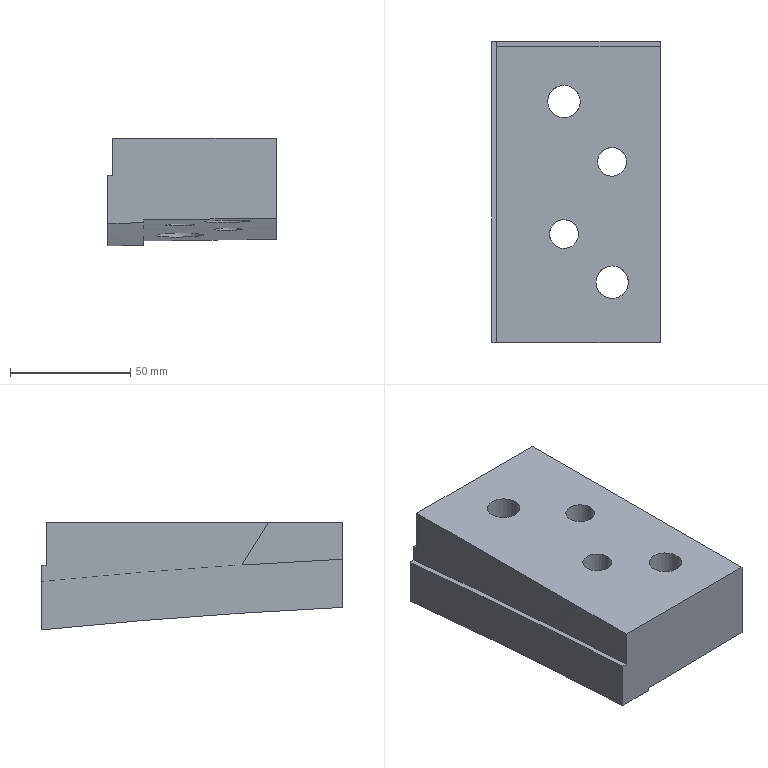Part | NX | features solid 2 | 1 solid | 20 faces | box 70 x 125 x 44.737 mm | volume 296261 mm3 | plane 9 | cylinder 6 | spline 5 | commonest cylinder face diameters 12 x2 13.5 x2 20 x2
STEP:
#1=CARTESIAN_POINT('',(-179.943,183.938,-35.287));
#2=VERTEX_POINT('',#1);
#3=CARTESIAN_POINT('',(-176.967,176.38,-34.573));
#4=CARTESIAN_POINT('',(-181.016,183.824,-35.305));
#5=CARTESIAN_POINT('',(-178.63,191.951,-35.933));
#6=CARTESIAN_POINT('',(-171.182,196.023,-36.198));
#7=CARTESIAN_POINT('',(-163.029,193.617,-35.866));
#8=CARTESIAN_POINT('',(-158.987,186.174,-35.195));
#9=CARTESIAN_POINT('',(-161.361,178.062,-34.509));
#10=CARTESIAN_POINT('',(-168.814,173.976,-34.242));
#11=CARTESIAN_POINT('',(-176.967,176.38,-34.573));
#12=CARTESIAN_POINT('',(-181.016,183.824,-35.305));
#13=CARTESIAN_POINT('',(-178.63,191.951,-35.933));
#14=B_SPLINE_CURVE_WITH_KNOTS('',3,(#3,#4,#5,#6,#7,#8,#9,#10,#11,#12,#13),.UNSPECIFIED.,.T.,.F.,(1,1,1,1,1,1,1,1,1,1,1,1,1,1,1),(-0.02349,-0.01566,-0.00783,0.,0.00783,0.01566,0.02349,0.03132,0.03915,0.04698,0.05481,0.06264,0.07047,0.0783,0.08613),.UNSPECIFIED.);
#15=EDGE_CURVE('',#2,#2,#14,.T.);
#16=ORIENTED_EDGE('',*,*,#15,.F.);
#17=EDGE_LOOP('',(#16));
#18=FACE_BOUND('',#17,.T.);
#19=CARTESIAN_POINT('',(-130.,85.,-28.186));
#20=VERTEX_POINT('',#19);
#21=CARTESIAN_POINT('',(-130.,210.,-36.981));
#22=VERTEX_POINT('',#21);
#23=CARTESIAN_POINT('',(-130.,85.,-28.186));
#24=CARTESIAN_POINT('',(-130.,90.217,-28.433));
#25=CARTESIAN_POINT('',(-130.,100.654,-28.855));
#26=CARTESIAN_POINT('',(-130.,113.697,-29.442));
#27=CARTESIAN_POINT('',(-130.,124.133,-29.882));
#28=CARTESIAN_POINT('',(-130.,131.938,-30.619));
#29=CARTESIAN_POINT('',(-130.,139.759,-31.08));
#30=CARTESIAN_POINT('',(-130.,147.597,-31.331));
#31=CARTESIAN_POINT('',(-130.,155.384,-32.198));
#32=CARTESIAN_POINT('',(-130.,163.186,-32.88));
#33=CARTESIAN_POINT('',(-130.,170.992,-33.525));
#34=CARTESIAN_POINT('',(-130.,181.393,-34.457));
#35=CARTESIAN_POINT('',(-130.,194.4,-35.557));
#36=CARTESIAN_POINT('',(-130.,204.797,-36.538));
#37=CARTESIAN_POINT('',(-130.,210.,-36.981));
#38=B_SPLINE_CURVE_WITH_KNOTS('',3,(#23,#24,#25,#26,#27,#28,#29,#30,#31,#32,#33,#34,#35,#36,#37),.UNSPECIFIED.,.F.,.F.,(4,1,1,1,1,1,1,1,1,1,1,1,4),(0.,0.01567,0.03134,0.03917,0.047,0.05484,0.06267,0.07051,0.07834,0.08617,0.09401,0.1097,0.1253),.UNSPECIFIED.);
#39=EDGE_CURVE('',#20,#22,#38,.T.);
#40=ORIENTED_EDGE('',*,*,#39,.F.);
#41=CARTESIAN_POINT('',(-185.066,85.,-28.984));
#42=VERTEX_POINT('',#41);
#43=CARTESIAN_POINT('',(-185.066,85.,-28.984));
#44=CARTESIAN_POINT('',(-166.712,85.,-28.666));
#45=CARTESIAN_POINT('',(-148.356,85.,-28.396));
#46=CARTESIAN_POINT('',(-130.,85.,-28.186));
#47=B_SPLINE_CURVE_WITH_KNOTS('',3,(#43,#44,#45,#46),.UNSPECIFIED.,.F.,.F.,(4,4),(0.,0.05507),.UNSPECIFIED.);
#48=EDGE_CURVE('',#42,#20,#47,.T.);
#49=ORIENTED_EDGE('',*,*,#48,.F.);
#50=CARTESIAN_POINT('',(-185.059,210.,-37.712));
#51=VERTEX_POINT('',#50);
#52=CARTESIAN_POINT('',(-185.059,210.,-37.712));
#53=CARTESIAN_POINT('',(-185.059,204.796,-37.285));
#54=CARTESIAN_POINT('',(-185.06,197.011,-36.442));
#55=CARTESIAN_POINT('',(-185.06,186.606,-35.6));
#56=CARTESIAN_POINT('',(-185.061,178.806,-34.92));
#57=CARTESIAN_POINT('',(-185.061,171.008,-34.212));
#58=CARTESIAN_POINT('',(-185.062,163.206,-33.565));
#59=CARTESIAN_POINT('',(-185.062,155.404,-32.91));
#60=CARTESIAN_POINT('',(-185.063,148.917,-32.201));
#61=CARTESIAN_POINT('',(-185.063,143.701,-31.915));
#62=CARTESIAN_POINT('',(-185.063,139.78,-31.878));
#63=CARTESIAN_POINT('',(-185.063,135.862,-31.76));
#64=CARTESIAN_POINT('',(-185.064,130.652,-31.347));
#65=CARTESIAN_POINT('',(-185.064,124.146,-30.694));
#66=CARTESIAN_POINT('',(-185.064,116.319,-30.312));
#67=CARTESIAN_POINT('',(-185.065,108.489,-29.983));
#68=CARTESIAN_POINT('',(-185.065,98.05,-29.531));
#69=CARTESIAN_POINT('',(-185.066,90.218,-29.244));
#70=CARTESIAN_POINT('',(-185.066,85.,-28.984));
#71=B_SPLINE_CURVE_WITH_KNOTS('',3,(#52,#53,#54,#55,#56,#57,#58,#59,#60,#61,#62,#63,#64,#65,#66,#67,#68,#69,#70),.UNSPECIFIED.,.F.,.F.,(4,1,1,1,1,1,1,1,1,1,1,1,1,1,1,1,4),(0.1412,0.1569,0.1647,0.1726,0.1804,0.1882,0.196,0.2039,0.2078,0.2117,0.2156,0.2195,0.2273,0.2352,0.243,0.2508,0.2665),.UNSPECIFIED.);
#72=EDGE_CURVE('',#51,#42,#71,.T.);
#73=ORIENTED_EDGE('',*,*,#72,.F.);
#74=CARTESIAN_POINT('',(-130.,210.,-36.981));
#75=CARTESIAN_POINT('',(-148.354,210.,-37.164));
#76=CARTESIAN_POINT('',(-166.707,210.,-37.411));
#77=CARTESIAN_POINT('',(-185.059,210.,-37.712));
#78=B_SPLINE_CURVE_WITH_KNOTS('',3,(#74,#75,#76,#77),.UNSPECIFIED.,.F.,.F.,(4,4),(0.007875,0.06294),.UNSPECIFIED.);
#79=EDGE_CURVE('',#22,#51,#78,.T.);
#80=ORIENTED_EDGE('',*,*,#79,.F.);
#81=EDGE_LOOP('',(#40,#49,#73,#80));
#82=FACE_BOUND('',#81,.T.);
#83=CARTESIAN_POINT('',(-144.006,159.739,-32.722));
#84=VERTEX_POINT('',#83);
#85=CARTESIAN_POINT('',(-145.504,155.098,-32.309));
#86=CARTESIAN_POINT('',(-143.359,159.713,-32.721));
#87=CARTESIAN_POINT('',(-145.094,164.485,-33.138));
#88=CARTESIAN_POINT('',(-149.702,166.645,-33.372));
#89=CARTESIAN_POINT('',(-154.499,164.9,-33.28));
#90=CARTESIAN_POINT('',(-156.639,160.284,-32.927));
#91=CARTESIAN_POINT('',(-154.91,155.521,-32.465));
#92=CARTESIAN_POINT('',(-150.302,153.354,-32.183));
#93=CARTESIAN_POINT('',(-145.504,155.098,-32.309));
#94=CARTESIAN_POINT('',(-143.359,159.713,-32.721));
#95=CARTESIAN_POINT('',(-145.094,164.485,-33.138));
#96=B_SPLINE_CURVE_WITH_KNOTS('',3,(#85,#86,#87,#88,#89,#90,#91,#92,#93,#94,#95),.UNSPECIFIED.,.T.,.F.,(1,1,1,1,1,1,1,1,1,1,1,1,1,1,1),(-0.0141,-0.009397,-0.004698,0.,0.004698,0.009397,0.0141,0.01879,0.02349,0.02819,0.03289,0.03759,0.04229,0.04698,0.05168),.UNSPECIFIED.);
#97=EDGE_CURVE('',#84,#84,#96,.T.);
#98=ORIENTED_EDGE('',*,*,#97,.T.);
#99=EDGE_LOOP('',(#98));
#100=FACE_BOUND('',#99,.T.);
#101=CARTESIAN_POINT('',(-164.006,129.731,-30.876));
#102=VERTEX_POINT('',#101);
#103=CARTESIAN_POINT('',(-165.511,125.091,-30.492));
#104=CARTESIAN_POINT('',(-163.359,129.705,-30.865));
#105=CARTESIAN_POINT('',(-165.087,134.477,-31.306));
#106=CARTESIAN_POINT('',(-169.692,136.644,-31.493));
#107=CARTESIAN_POINT('',(-174.491,134.907,-31.495));
#108=CARTESIAN_POINT('',(-176.639,130.294,-31.149));
#109=CARTESIAN_POINT('',(-174.918,125.53,-30.677));
#110=CARTESIAN_POINT('',(-170.312,123.355,-30.46));
#111=CARTESIAN_POINT('',(-165.511,125.091,-30.492));
#112=CARTESIAN_POINT('',(-163.359,129.705,-30.865));
#113=CARTESIAN_POINT('',(-165.087,134.477,-31.306));
#114=B_SPLINE_CURVE_WITH_KNOTS('',3,(#103,#104,#105,#106,#107,#108,#109,#110,#111,#112,#113),.UNSPECIFIED.,.T.,.F.,(1,1,1,1,1,1,1,1,1,1,1,1,1,1,1),(-0.01409,-0.009395,-0.004697,0.,0.004697,0.009395,0.01409,0.01879,0.02349,0.02818,0.03288,0.03758,0.04228,0.04697,0.05167),.UNSPECIFIED.);
#115=EDGE_CURVE('',#102,#102,#114,.T.);
#116=ORIENTED_EDGE('',*,*,#115,.T.);
#117=EDGE_LOOP('',(#116));
#118=FACE_BOUND('',#117,.T.);
#119=CARTESIAN_POINT('',(-159.944,108.946,-29.606));
#120=VERTEX_POINT('',#119);
#121=CARTESIAN_POINT('',(-156.963,101.377,-29.24));
#122=CARTESIAN_POINT('',(-161.021,108.833,-29.617));
#123=CARTESIAN_POINT('',(-158.617,116.966,-29.93));
#124=CARTESIAN_POINT('',(-151.174,121.019,-30.029));
#125=CARTESIAN_POINT('',(-143.034,118.62,-29.799));
#126=CARTESIAN_POINT('',(-138.983,111.17,-29.425));
#127=CARTESIAN_POINT('',(-141.372,103.047,-29.105));
#128=CARTESIAN_POINT('',(-148.822,98.979,-29.022));
#129=CARTESIAN_POINT('',(-156.963,101.377,-29.24));
#130=CARTESIAN_POINT('',(-161.021,108.833,-29.617));
#131=CARTESIAN_POINT('',(-158.617,116.966,-29.93));
#132=B_SPLINE_CURVE_WITH_KNOTS('',3,(#121,#122,#123,#124,#125,#126,#127,#128,#129,#130,#131),.UNSPECIFIED.,.T.,.F.,(1,1,1,1,1,1,1,1,1,1,1,1,1,1,1),(-0.02346,-0.01564,-0.007819,0.,0.007819,0.01564,0.02346,0.03128,0.0391,0.04692,0.05473,0.06255,0.07037,0.07819,0.08601),.UNSPECIFIED.);
#133=EDGE_CURVE('',#120,#120,#132,.T.);
#134=ORIENTED_EDGE('',*,*,#133,.F.);
#135=EDGE_LOOP('',(#134));
#136=FACE_BOUND('',#135,.T.);
#137=CARTESIAN_POINT('',(-125.164,210.,-36.934));
#138=CARTESIAN_POINT('',(-125.138,208.227,-36.783));
#139=CARTESIAN_POINT('',(-125.034,203.794,-36.406));
#140=CARTESIAN_POINT('',(-125.103,195.358,-35.605));
#141=CARTESIAN_POINT('',(-125.804,184.682,-34.716));
#142=CARTESIAN_POINT('',(-125.853,174.009,-33.744));
#143=CARTESIAN_POINT('',(-126.739,164.665,-32.97));
#144=CARTESIAN_POINT('',(-126.764,155.367,-32.181));
#145=CARTESIAN_POINT('',(-124.796,145.924,-31.099));
#146=CARTESIAN_POINT('',(-129.204,135.731,-30.995));
#147=CARTESIAN_POINT('',(-128.429,126.264,-29.981));
#148=CARTESIAN_POINT('',(-128.955,115.603,-29.504));
#149=CARTESIAN_POINT('',(-129.112,106.237,-29.102));
#150=CARTESIAN_POINT('',(-129.396,95.595,-28.637));
#151=CARTESIAN_POINT('',(-129.537,88.96,-28.368));
#152=CARTESIAN_POINT('',(-129.631,85.,-28.182));
#153=CARTESIAN_POINT('',(-130.684,210.,-36.986));
#154=CARTESIAN_POINT('',(-130.661,208.227,-36.835));
#155=CARTESIAN_POINT('',(-130.564,203.794,-36.459));
#156=CARTESIAN_POINT('',(-130.648,195.358,-35.651));
#157=CARTESIAN_POINT('',(-131.356,184.682,-34.768));
#158=CARTESIAN_POINT('',(-131.419,174.009,-33.796));
#159=CARTESIAN_POINT('',(-132.305,164.665,-33.02));
#160=CARTESIAN_POINT('',(-132.34,155.367,-32.235));
#161=CARTESIAN_POINT('',(-130.411,145.924,-31.149));
#162=CARTESIAN_POINT('',(-134.764,135.731,-31.07));
#163=CARTESIAN_POINT('',(-134.01,126.264,-30.045));
#164=CARTESIAN_POINT('',(-134.538,115.603,-29.561));
#165=CARTESIAN_POINT('',(-134.701,106.237,-29.163));
#166=CARTESIAN_POINT('',(-134.989,95.595,-28.699));
#167=CARTESIAN_POINT('',(-135.133,88.96,-28.432));
#168=CARTESIAN_POINT('',(-135.229,85.,-28.246));
#169=CARTESIAN_POINT('',(-151.145,210.,-37.199));
#170=CARTESIAN_POINT('',(-151.132,208.227,-37.049));
#171=CARTESIAN_POINT('',(-151.065,203.794,-36.675));
#172=CARTESIAN_POINT('',(-151.203,195.358,-35.837));
#173=CARTESIAN_POINT('',(-151.935,184.682,-34.977));
#174=CARTESIAN_POINT('',(-152.049,174.009,-34.003));
#175=CARTESIAN_POINT('',(-152.939,164.665,-33.223));
#176=CARTESIAN_POINT('',(-153.012,155.367,-32.456));
#177=CARTESIAN_POINT('',(-151.223,145.924,-31.351));
#178=CARTESIAN_POINT('',(-155.373,135.731,-31.368));
#179=CARTESIAN_POINT('',(-154.699,126.264,-30.304));
#180=CARTESIAN_POINT('',(-155.234,115.603,-29.795));
#181=CARTESIAN_POINT('',(-155.417,106.237,-29.41));
#182=CARTESIAN_POINT('',(-155.724,95.595,-28.948));
#183=CARTESIAN_POINT('',(-155.877,88.96,-28.69));
#184=CARTESIAN_POINT('',(-155.978,85.,-28.501));
#185=CARTESIAN_POINT('',(-171.603,210.,-37.489));
#186=CARTESIAN_POINT('',(-171.602,208.227,-37.342));
#187=CARTESIAN_POINT('',(-171.565,203.794,-36.974));
#188=CARTESIAN_POINT('',(-171.758,195.358,-36.088));
#189=CARTESIAN_POINT('',(-172.514,184.682,-35.254));
#190=CARTESIAN_POINT('',(-172.68,174.009,-34.276));
#191=CARTESIAN_POINT('',(-173.573,164.665,-33.491));
#192=CARTESIAN_POINT('',(-173.683,155.367,-32.745));
#193=CARTESIAN_POINT('',(-172.035,145.924,-31.619));
#194=CARTESIAN_POINT('',(-175.982,135.731,-31.747));
#195=CARTESIAN_POINT('',(-175.387,126.264,-30.641));
#196=CARTESIAN_POINT('',(-175.929,115.603,-30.109));
#197=CARTESIAN_POINT('',(-176.133,106.237,-29.735));
#198=CARTESIAN_POINT('',(-176.457,95.595,-29.273));
#199=CARTESIAN_POINT('',(-176.619,88.96,-29.027));
#200=CARTESIAN_POINT('',(-176.727,85.,-28.833));
#201=CARTESIAN_POINT('',(-186.542,210.,-37.737));
#202=CARTESIAN_POINT('',(-186.549,208.227,-37.591));
#203=CARTESIAN_POINT('',(-186.534,203.794,-37.227));
#204=CARTESIAN_POINT('',(-186.766,195.358,-36.317));
#205=CARTESIAN_POINT('',(-187.54,184.682,-35.497));
#206=CARTESIAN_POINT('',(-187.743,174.009,-34.519));
#207=CARTESIAN_POINT('',(-188.638,164.665,-33.732));
#208=CARTESIAN_POINT('',(-188.776,155.367,-32.999));
#209=CARTESIAN_POINT('',(-187.231,145.924,-31.866));
#210=CARTESIAN_POINT('',(-191.029,135.731,-32.045));
#211=CARTESIAN_POINT('',(-190.493,126.264,-30.916));
#212=CARTESIAN_POINT('',(-191.04,115.603,-30.37));
#213=CARTESIAN_POINT('',(-191.259,106.237,-30.002));
#214=CARTESIAN_POINT('',(-191.596,95.595,-29.541));
#215=CARTESIAN_POINT('',(-191.765,88.96,-29.301));
#216=CARTESIAN_POINT('',(-191.877,85.,-29.103));
#217=B_SPLINE_SURFACE_WITH_KNOTS('',3,3,((#137,#138,#139,#140,#141,#142,#143,#144,#145,#146,#147,#148,#149,#150,#151,#152),(#153,#154,#155,#156,#157,#158,#159,#160,#161,#162,#163,#164,#165,#166,#167,#168),(#169,#170,#171,#172,#173,#174,#175,#176,#177,#178,#179,#180,#181,#182,#183,#184),(#185,#186,#187,#188,#189,#190,#191,#192,#193,#194,#195,#196,#197,#198,#199,#200),(#201,#202,#203,#204,#205,#206,#207,#208,#209,#210,#211,#212,#213,#214,#215,#216)),.UNSPECIFIED.,.F.,.F.,.F.,(4,1,4),(4,1,1,1,1,1,1,1,1,1,1,1,1,4),(0.6105,0.625,0.6643),(0.5208,0.5312,0.5469,0.5703,0.5938,0.6094,0.625,0.6484,0.6641,0.6875,0.7031,0.7266,0.7422,0.7653),.UNSPECIFIED.);
#218=ADVANCED_FACE('',(#18,#82,#100,#118,#136),#217,.F.);
#219=CARTESIAN_POINT('',(-198.,210.,-13.));
#220=VERTEX_POINT('',#219);
#221=CARTESIAN_POINT('',(-130.,210.,-13.));
#222=VERTEX_POINT('',#221);
#223=CARTESIAN_POINT('',(-198.,210.,-13.));
#224=DIRECTION('',(1.,0.,0.));
#225=VECTOR('',#224,1000.);
#226=LINE('',#223,#225);
#227=EDGE_CURVE('',#220,#222,#226,.T.);
#228=ORIENTED_EDGE('',*,*,#227,.T.);
#229=CARTESIAN_POINT('',(-130.,210.,2.));
#230=DIRECTION('',(0.,0.,1.));
#231=VECTOR('',#230,1000.);
#232=LINE('',#229,#231);
#233=EDGE_CURVE('',#22,#222,#232,.T.);
#234=ORIENTED_EDGE('',*,*,#233,.F.);
#235=ORIENTED_EDGE('',*,*,#79,.T.);
#236=CARTESIAN_POINT('',(-185.059,210.,-39.489));
#237=VERTEX_POINT('',#236);
#238=CARTESIAN_POINT('',(-185.059,210.,-115.));
#239=DIRECTION('',(0.,0.,-1.));
#240=VECTOR('',#239,1000.);
#241=LINE('',#238,#240);
#242=EDGE_CURVE('',#51,#237,#241,.T.);
#243=ORIENTED_EDGE('',*,*,#242,.T.);
#244=CARTESIAN_POINT('',(-200.,210.,-39.737));
#245=VERTEX_POINT('',#244);
#246=CARTESIAN_POINT('',(-200.,210.,-39.737));
#247=CARTESIAN_POINT('',(-195.02,210.,-39.651));
#248=CARTESIAN_POINT('',(-190.039,210.,-39.568));
#249=CARTESIAN_POINT('',(-185.059,210.,-39.489));
#250=B_SPLINE_CURVE_WITH_KNOTS('',3,(#246,#247,#248,#249),.UNSPECIFIED.,.F.,.F.,(4,4),(0.000111,0.01505),.UNSPECIFIED.);
#251=EDGE_CURVE('',#245,#237,#250,.T.);
#252=ORIENTED_EDGE('',*,*,#251,.F.);
#253=CARTESIAN_POINT('',(-200.,210.,-19.737));
#254=VERTEX_POINT('',#253);
#255=CARTESIAN_POINT('',(-200.,210.,-34.243));
#256=DIRECTION('',(0.,0.,1.));
#257=VECTOR('',#256,1000.);
#258=LINE('',#255,#257);
#259=EDGE_CURVE('',#254,#245,#258,.F.);
#260=ORIENTED_EDGE('',*,*,#259,.F.);
#261=CARTESIAN_POINT('',(-198.,210.,-19.737));
#262=VERTEX_POINT('',#261);
#263=CARTESIAN_POINT('',(-200.,210.,-19.737));
#264=CARTESIAN_POINT('',(-199.333,210.,-19.737));
#265=CARTESIAN_POINT('',(-198.667,210.,-19.737));
#266=CARTESIAN_POINT('',(-198.,210.,-19.737));
#267=B_SPLINE_CURVE_WITH_KNOTS('',3,(#263,#264,#265,#266),.UNSPECIFIED.,.F.,.F.,(4,4),(0.00001231,0.002012),.UNSPECIFIED.);
#268=EDGE_CURVE('',#254,#262,#267,.T.);
#269=ORIENTED_EDGE('',*,*,#268,.T.);
#270=CARTESIAN_POINT('',(-198.,210.,2.806));
#271=DIRECTION('',(0.,0.,1.));
#272=VECTOR('',#271,1000.);
#273=LINE('',#270,#272);
#274=EDGE_CURVE('',#262,#220,#273,.T.);
#275=ORIENTED_EDGE('',*,*,#274,.T.);
#276=EDGE_LOOP('',(#228,#234,#235,#243,#252,#260,#269,#275));
#277=FACE_BOUND('',#276,.T.);
#278=CARTESIAN_POINT('',(130.,210.,-37.085));
#279=DIRECTION('',(0.,1.,0.));
#280=DIRECTION('',(0.,0.,1.));
#281=AXIS2_PLACEMENT_3D('',#278,#279,#280);
#282=PLANE('',#281);
#283=ADVANCED_FACE('',(#277),#282,.T.);
#284=CARTESIAN_POINT('',(-130.,85.,5.));
#285=VERTEX_POINT('',#284);
#286=CARTESIAN_POINT('',(-198.,85.,5.));
#287=VERTEX_POINT('',#286);
#288=CARTESIAN_POINT('',(412.414,85.,5.));
#289=DIRECTION('',(-1.,0.,0.));
#290=VECTOR('',#289,1000.);
#291=LINE('',#288,#290);
#292=EDGE_CURVE('',#285,#287,#291,.T.);
#293=ORIENTED_EDGE('',*,*,#292,.T.);
#294=CARTESIAN_POINT('',(-198.,85.,-10.4));
#295=VERTEX_POINT('',#294);
#296=CARTESIAN_POINT('',(-198.,85.,229.6));
#297=DIRECTION('',(0.,0.,1.));
#298=VECTOR('',#297,1000.);
#299=LINE('',#296,#298);
#300=EDGE_CURVE('',#287,#295,#299,.F.);
#301=ORIENTED_EDGE('',*,*,#300,.T.);
#302=CARTESIAN_POINT('',(-200.,85.,-10.4));
#303=VERTEX_POINT('',#302);
#304=CARTESIAN_POINT('',(-198.,85.,-10.4));
#305=CARTESIAN_POINT('',(-198.667,85.,-10.4));
#306=CARTESIAN_POINT('',(-199.333,85.,-10.4));
#307=CARTESIAN_POINT('',(-200.,85.,-10.4));
#308=B_SPLINE_CURVE_WITH_KNOTS('',3,(#304,#305,#306,#307),.UNSPECIFIED.,.F.,.F.,(4,4),(0.,1.),.UNSPECIFIED.);
#309=EDGE_CURVE('',#303,#295,#308,.F.);
#310=ORIENTED_EDGE('',*,*,#309,.F.);
#311=CARTESIAN_POINT('',(-200.,85.,-30.4));
#312=VERTEX_POINT('',#311);
#313=CARTESIAN_POINT('',(-200.,85.,-36.84));
#314=DIRECTION('',(0.,0.,1.));
#315=VECTOR('',#314,1000.);
#316=LINE('',#313,#315);
#317=EDGE_CURVE('',#303,#312,#316,.F.);
#318=ORIENTED_EDGE('',*,*,#317,.T.);
#319=CARTESIAN_POINT('',(-185.066,85.,-30.16));
#320=VERTEX_POINT('',#319);
#321=CARTESIAN_POINT('',(-200.,85.,-30.4));
#322=CARTESIAN_POINT('',(-195.022,85.,-30.317));
#323=CARTESIAN_POINT('',(-190.044,85.,-30.237));
#324=CARTESIAN_POINT('',(-185.066,85.,-30.16));
#325=B_SPLINE_CURVE_WITH_KNOTS('',3,(#321,#322,#323,#324),.UNSPECIFIED.,.F.,.F.,(4,4),(0.0001508,0.01509),.UNSPECIFIED.);
#326=EDGE_CURVE('',#312,#320,#325,.T.);
#327=ORIENTED_EDGE('',*,*,#326,.T.);
#328=CARTESIAN_POINT('',(-185.066,85.,-115.));
#329=DIRECTION('',(0.,0.,-1.));
#330=VECTOR('',#329,1000.);
#331=LINE('',#328,#330);
#332=EDGE_CURVE('',#42,#320,#331,.T.);
#333=ORIENTED_EDGE('',*,*,#332,.F.);
#334=ORIENTED_EDGE('',*,*,#48,.T.);
#335=CARTESIAN_POINT('',(-130.,85.,0.505));
#336=DIRECTION('',(0.,0.,-1.));
#337=VECTOR('',#336,1000.);
#338=LINE('',#335,#337);
#339=EDGE_CURVE('',#285,#20,#338,.T.);
#340=ORIENTED_EDGE('',*,*,#339,.F.);
#341=EDGE_LOOP('',(#293,#301,#310,#318,#327,#333,#334,#340));
#342=FACE_BOUND('',#341,.T.);
#343=CARTESIAN_POINT('',(412.414,85.,0.505));
#344=DIRECTION('',(0.,1.,0.));
#345=DIRECTION('',(0.,0.,1.));
#346=AXIS2_PLACEMENT_3D('',#343,#344,#345);
#347=PLANE('',#346);
#348=ADVANCED_FACE('',(#342),#347,.F.);
#349=CARTESIAN_POINT('',(-156.75,110.,5.));
#350=VERTEX_POINT('',#349);
#351=CARTESIAN_POINT('',(-150.,110.,5.));
#352=DIRECTION('',(0.,0.,-1.));
#353=DIRECTION('',(-1.,0.,0.));
#354=AXIS2_PLACEMENT_3D('',#351,#352,#353);
#355=CIRCLE('',#354,6.75);
#356=EDGE_CURVE('',#350,#350,#355,.F.);
#357=ORIENTED_EDGE('',*,*,#356,.F.);
#358=EDGE_LOOP('',(#357));
#359=FACE_BOUND('',#358,.T.);
#360=CARTESIAN_POINT('',(-176.,130.,5.));
#361=VERTEX_POINT('',#360);
#362=CARTESIAN_POINT('',(-170.,130.,5.));
#363=DIRECTION('',(0.,0.,-1.));
#364=DIRECTION('',(-1.,0.,0.));
#365=AXIS2_PLACEMENT_3D('',#362,#363,#364);
#366=CIRCLE('',#365,6.);
#367=EDGE_CURVE('',#361,#361,#366,.F.);
#368=ORIENTED_EDGE('',*,*,#367,.F.);
#369=EDGE_LOOP('',(#368));
#370=FACE_BOUND('',#369,.T.);
#371=CARTESIAN_POINT('',(-156.,160.,5.));
#372=VERTEX_POINT('',#371);
#373=CARTESIAN_POINT('',(-150.,160.,5.));
#374=DIRECTION('',(0.,0.,-1.));
#375=DIRECTION('',(-1.,0.,0.));
#376=AXIS2_PLACEMENT_3D('',#373,#374,#375);
#377=CIRCLE('',#376,6.);
#378=EDGE_CURVE('',#372,#372,#377,.F.);
#379=ORIENTED_EDGE('',*,*,#378,.F.);
#380=EDGE_LOOP('',(#379));
#381=FACE_BOUND('',#380,.T.);
#382=CARTESIAN_POINT('',(-176.75,185.,5.));
#383=VERTEX_POINT('',#382);
#384=CARTESIAN_POINT('',(-170.,185.,5.));
#385=DIRECTION('',(0.,0.,-1.));
#386=DIRECTION('',(-1.,0.,0.));
#387=AXIS2_PLACEMENT_3D('',#384,#385,#386);
#388=CIRCLE('',#387,6.75);
#389=EDGE_CURVE('',#383,#383,#388,.F.);
#390=ORIENTED_EDGE('',*,*,#389,.F.);
#391=EDGE_LOOP('',(#390));
#392=FACE_BOUND('',#391,.T.);
#393=CARTESIAN_POINT('',(-198.,208.,5.));
#394=VERTEX_POINT('',#393);
#395=CARTESIAN_POINT('',(-130.,208.,5.));
#396=VERTEX_POINT('',#395);
#397=CARTESIAN_POINT('',(-198.,208.,5.));
#398=DIRECTION('',(1.,0.,0.));
#399=VECTOR('',#398,1000.);
#400=LINE('',#397,#399);
#401=EDGE_CURVE('',#394,#396,#400,.T.);
#402=ORIENTED_EDGE('',*,*,#401,.F.);
#403=CARTESIAN_POINT('',(-198.,85.,5.));
#404=CARTESIAN_POINT('',(-197.999,126.,5.));
#405=CARTESIAN_POINT('',(-198.,167.,5.));
#406=CARTESIAN_POINT('',(-198.,208.,5.));
#407=B_SPLINE_CURVE_WITH_KNOTS('',3,(#403,#404,#405,#406),.UNSPECIFIED.,.F.,.F.,(4,4),(1.013,1.136),.UNSPECIFIED.);
#408=EDGE_CURVE('',#394,#287,#407,.F.);
#409=ORIENTED_EDGE('',*,*,#408,.T.);
#410=ORIENTED_EDGE('',*,*,#292,.F.);
#411=CARTESIAN_POINT('',(-130.,0.,5.));
#412=DIRECTION('',(0.,-1.,0.));
#413=VECTOR('',#412,1000.);
#414=LINE('',#411,#413);
#415=EDGE_CURVE('',#396,#285,#414,.T.);
#416=ORIENTED_EDGE('',*,*,#415,.F.);
#417=EDGE_LOOP('',(#402,#409,#410,#416));
#418=FACE_BOUND('',#417,.T.);
#419=CARTESIAN_POINT('',(0.,0.,5.));
#420=DIRECTION('',(0.,0.,1.));
#421=DIRECTION('',(-1.,0.,0.));
#422=AXIS2_PLACEMENT_3D('',#419,#420,#421);
#423=PLANE('',#422);
#424=ADVANCED_FACE('',(#359,#370,#381,#392,#418),#423,.T.);
#425=ORIENTED_EDGE('',*,*,#72,.T.);
#426=ORIENTED_EDGE('',*,*,#332,.T.);
#427=CARTESIAN_POINT('',(-185.059,210.,-39.489));
#428=CARTESIAN_POINT('',(-185.061,168.429,-35.293));
#429=CARTESIAN_POINT('',(-185.064,126.732,-32.197));
#430=CARTESIAN_POINT('',(-185.066,85.,-30.16));
#431=B_SPLINE_CURVE_WITH_KNOTS('',3,(#427,#428,#429,#430),.UNSPECIFIED.,.F.,.F.,(4,4),(0.2096,0.335),.UNSPECIFIED.);
#432=EDGE_CURVE('',#237,#320,#431,.T.);
#433=ORIENTED_EDGE('',*,*,#432,.F.);
#434=ORIENTED_EDGE('',*,*,#242,.F.);
#435=EDGE_LOOP('',(#425,#426,#433,#434));
#436=FACE_BOUND('',#435,.T.);
#437=CARTESIAN_POINT('',(-185.071,-2.633,-115.));
#438=DIRECTION('',(1.,-0.00005855,0.));
#439=DIRECTION('',(-0.00005855,-1.,0.));
#440=AXIS2_PLACEMENT_3D('',#437,#438,#439);
#441=PLANE('',#440);
#442=ADVANCED_FACE('',(#436),#441,.T.);
#443=ORIENTED_EDGE('',*,*,#251,.T.);
#444=ORIENTED_EDGE('',*,*,#432,.T.);
#445=ORIENTED_EDGE('',*,*,#326,.F.);
#446=CARTESIAN_POINT('',(-200.,85.,-30.4));
#447=CARTESIAN_POINT('',(-199.999,126.748,-32.44));
#448=CARTESIAN_POINT('',(-200.,168.419,-35.536));
#449=CARTESIAN_POINT('',(-200.,210.,-39.737));
#450=B_SPLINE_CURVE_WITH_KNOTS('',3,(#446,#447,#448,#449),.UNSPECIFIED.,.F.,.F.,(4,4),(0.06314,0.1885),.UNSPECIFIED.);
#451=EDGE_CURVE('',#312,#245,#450,.T.);
#452=ORIENTED_EDGE('',*,*,#451,.T.);
#453=EDGE_LOOP('',(#443,#444,#445,#452));
#454=FACE_BOUND('',#453,.T.);
#455=CARTESIAN_POINT('',(-200.09,210.782,-39.817));
#456=CARTESIAN_POINT('',(-196.307,210.774,-39.751));
#457=CARTESIAN_POINT('',(-192.525,210.766,-39.687));
#458=CARTESIAN_POINT('',(-188.743,210.759,-39.624));
#459=CARTESIAN_POINT('',(-184.961,210.752,-39.564));
#460=CARTESIAN_POINT('',(-200.093,179.075,-36.604));
#461=CARTESIAN_POINT('',(-196.311,179.067,-36.538));
#462=CARTESIAN_POINT('',(-192.529,179.06,-36.475));
#463=CARTESIAN_POINT('',(-188.746,179.052,-36.413));
#464=CARTESIAN_POINT('',(-184.964,179.045,-36.353));
#465=CARTESIAN_POINT('',(-200.097,147.424,-33.968));
#466=CARTESIAN_POINT('',(-196.315,147.416,-33.904));
#467=CARTESIAN_POINT('',(-192.532,147.409,-33.841));
#468=CARTESIAN_POINT('',(-188.75,147.402,-33.779));
#469=CARTESIAN_POINT('',(-184.967,147.394,-33.72));
#470=CARTESIAN_POINT('',(-200.101,115.819,-31.898));
#471=CARTESIAN_POINT('',(-196.319,115.812,-31.834));
#472=CARTESIAN_POINT('',(-192.536,115.804,-31.771));
#473=CARTESIAN_POINT('',(-188.754,115.797,-31.711));
#474=CARTESIAN_POINT('',(-184.971,115.79,-31.652));
#475=CARTESIAN_POINT('',(-200.107,84.252,-30.366));
#476=CARTESIAN_POINT('',(-196.325,84.244,-30.302));
#477=CARTESIAN_POINT('',(-192.542,84.237,-30.24));
#478=CARTESIAN_POINT('',(-188.759,84.23,-30.18));
#479=CARTESIAN_POINT('',(-184.977,84.223,-30.121));
#480=B_SPLINE_SURFACE_WITH_KNOTS('',4,4,((#455,#456,#457,#458,#459),(#460,#461,#462,#463,#464),(#465,#466,#467,#468,#469),(#470,#471,#472,#473,#474),(#475,#476,#477,#478,#479)),.UNSPECIFIED.,.F.,.F.,.F.,(5,5),(5,5),(0.517,0.7098),(0.5564,0.5748),.PIECEWISE_BEZIER_KNOTS.);
#481=ADVANCED_FACE('',(#454),#480,.F.);
#482=CARTESIAN_POINT('',(-200.,85.,-10.4));
#483=CARTESIAN_POINT('',(-199.999,126.738,-12.439));
#484=CARTESIAN_POINT('',(-200.,168.424,-15.537));
#485=CARTESIAN_POINT('',(-200.,210.,-19.737));
#486=B_SPLINE_CURVE_WITH_KNOTS('',3,(#482,#483,#484,#485),.UNSPECIFIED.,.F.,.F.,(4,4),(0.,0.1254),.UNSPECIFIED.);
#487=EDGE_CURVE('',#303,#254,#486,.T.);
#488=ORIENTED_EDGE('',*,*,#487,.F.);
#489=ORIENTED_EDGE('',*,*,#309,.T.);
#490=CARTESIAN_POINT('',(-198.,210.,-19.737));
#491=CARTESIAN_POINT('',(-198.,168.419,-15.537));
#492=CARTESIAN_POINT('',(-197.999,126.751,-12.44));
#493=CARTESIAN_POINT('',(-198.,85.,-10.4));
#494=B_SPLINE_CURVE_WITH_KNOTS('',3,(#490,#491,#492,#493),.UNSPECIFIED.,.F.,.F.,(4,4),(0.5298,1.),.UNSPECIFIED.);
#495=EDGE_CURVE('',#295,#262,#494,.F.);
#496=ORIENTED_EDGE('',*,*,#495,.T.);
#497=ORIENTED_EDGE('',*,*,#268,.F.);
#498=EDGE_LOOP('',(#488,#489,#496,#497));
#499=FACE_BOUND('',#498,.T.);
#500=CARTESIAN_POINT('',(-198.,85.,-10.4));
#501=CARTESIAN_POINT('',(-197.999,126.751,-12.44));
#502=CARTESIAN_POINT('',(-198.,168.419,-15.537));
#503=CARTESIAN_POINT('',(-198.,210.,-19.737));
#504=CARTESIAN_POINT('',(-200.,85.,-10.4));
#505=CARTESIAN_POINT('',(-199.999,126.751,-12.44));
#506=CARTESIAN_POINT('',(-200.,168.419,-15.537));
#507=CARTESIAN_POINT('',(-200.,210.,-19.737));
#508=CARTESIAN_POINT('',(-200.012,85.,-10.4));
#509=CARTESIAN_POINT('',(-200.012,126.751,-12.44));
#510=CARTESIAN_POINT('',(-200.012,168.419,-15.537));
#511=CARTESIAN_POINT('',(-200.012,210.,-19.737));
#512=B_SPLINE_SURFACE_WITH_KNOTS('',1,3,((#500,#501,#502,#503),(#504,#505,#506,#507),(#508,#509,#510,#511)),.RULED_SURF.,.F.,.F.,.F.,(2,1,2),(4,4),(0.,1.,1.006),(0.,0.4702),.PIECEWISE_BEZIER_KNOTS.);
#513=ADVANCED_FACE('',(#499),#512,.F.);
#514=ORIENTED_EDGE('',*,*,#259,.T.);
#515=ORIENTED_EDGE('',*,*,#451,.F.);
#516=ORIENTED_EDGE('',*,*,#317,.F.);
#517=ORIENTED_EDGE('',*,*,#487,.T.);
#518=EDGE_LOOP('',(#514,#515,#516,#517));
#519=FACE_BOUND('',#518,.T.);
#520=CARTESIAN_POINT('',(-200.,210.,-39.913));
#521=CARTESIAN_POINT('',(-200.,210.,-10.224));
#522=CARTESIAN_POINT('',(-200.,168.333,-39.913));
#523=CARTESIAN_POINT('',(-200.,168.333,-10.224));
#524=CARTESIAN_POINT('',(-199.999,126.667,-39.913));
#525=CARTESIAN_POINT('',(-199.999,126.667,-10.224));
#526=CARTESIAN_POINT('',(-200.,85.,-39.913));
#527=CARTESIAN_POINT('',(-200.,85.,-10.224));
#528=B_SPLINE_SURFACE_WITH_KNOTS('',3,1,((#520,#521),(#522,#523),(#524,#525),(#526,#527)),.SURF_OF_LINEAR_EXTRUSION.,.F.,.F.,.F.,(4,4),(2,2),(0.8605,0.9303),(0.,1.),.PIECEWISE_BEZIER_KNOTS.);
#529=ADVANCED_FACE('',(#519),#528,.T.);
#530=CARTESIAN_POINT('',(-198.,208.,-13.));
#531=VERTEX_POINT('',#530);
#532=CARTESIAN_POINT('',(-198.,210.,-13.));
#533=DIRECTION('',(0.,-1.,0.));
#534=VECTOR('',#533,1000.);
#535=LINE('',#532,#534);
#536=EDGE_CURVE('',#220,#531,#535,.T.);
#537=ORIENTED_EDGE('',*,*,#536,.F.);
#538=ORIENTED_EDGE('',*,*,#274,.F.);
#539=ORIENTED_EDGE('',*,*,#495,.F.);
#540=ORIENTED_EDGE('',*,*,#300,.F.);
#541=ORIENTED_EDGE('',*,*,#408,.F.);
#542=CARTESIAN_POINT('',(-198.,208.,7.));
#543=DIRECTION('',(0.,0.,-1.));
#544=VECTOR('',#543,1000.);
#545=LINE('',#542,#544);
#546=EDGE_CURVE('',#394,#531,#545,.T.);
#547=ORIENTED_EDGE('',*,*,#546,.T.);
#548=EDGE_LOOP('',(#537,#538,#539,#540,#541,#547));
#549=FACE_BOUND('',#548,.T.);
#550=CARTESIAN_POINT('',(-198.,85.,-10.4));
#551=CARTESIAN_POINT('',(-198.,85.,14.282));
#552=CARTESIAN_POINT('',(-197.999,126.999,-12.452));
#553=CARTESIAN_POINT('',(-197.999,126.999,12.231));
#554=CARTESIAN_POINT('',(-198.,168.919,-15.573));
#555=CARTESIAN_POINT('',(-198.,168.919,9.109));
#556=CARTESIAN_POINT('',(-198.,210.748,-19.812));
#557=CARTESIAN_POINT('',(-198.,210.748,4.87));
#558=B_SPLINE_SURFACE_WITH_KNOTS('',3,1,((#550,#551),(#552,#553),(#554,#555),(#556,#557)),.SURF_OF_LINEAR_EXTRUSION.,.F.,.F.,.F.,(4,4),(2,2),(0.,0.473),(0.,1.),.PIECEWISE_BEZIER_KNOTS.);
#559=ADVANCED_FACE('',(#549),#558,.F.);
#560=CARTESIAN_POINT('',(-130.,208.,-13.));
#561=VERTEX_POINT('',#560);
#562=CARTESIAN_POINT('',(-130.,208.,7.));
#563=DIRECTION('',(0.,0.,-1.));
#564=VECTOR('',#563,1000.);
#565=LINE('',#562,#564);
#566=EDGE_CURVE('',#396,#561,#565,.T.);
#567=ORIENTED_EDGE('',*,*,#566,.F.);
#568=ORIENTED_EDGE('',*,*,#415,.T.);
#569=ORIENTED_EDGE('',*,*,#339,.T.);
#570=ORIENTED_EDGE('',*,*,#39,.T.);
#571=ORIENTED_EDGE('',*,*,#233,.T.);
#572=CARTESIAN_POINT('',(-130.,210.,-13.));
#573=DIRECTION('',(0.,-1.,0.));
#574=VECTOR('',#573,1000.);
#575=LINE('',#572,#574);
#576=EDGE_CURVE('',#222,#561,#575,.T.);
#577=ORIENTED_EDGE('',*,*,#576,.T.);
#578=EDGE_LOOP('',(#567,#568,#569,#570,#571,#577));
#579=FACE_BOUND('',#578,.T.);
#580=CARTESIAN_POINT('',(-130.,0.,2.));
#581=DIRECTION('',(-1.,0.,0.));
#582=DIRECTION('',(0.,0.,-1.));
#583=AXIS2_PLACEMENT_3D('',#580,#581,#582);
#584=PLANE('',#583);
#585=ADVANCED_FACE('',(#579),#584,.F.);
#586=ORIENTED_EDGE('',*,*,#576,.F.);
#587=ORIENTED_EDGE('',*,*,#227,.F.);
#588=ORIENTED_EDGE('',*,*,#536,.T.);
#589=CARTESIAN_POINT('',(-198.,208.,-13.));
#590=DIRECTION('',(-1.,0.,0.));
#591=VECTOR('',#590,1000.);
#592=LINE('',#589,#591);
#593=EDGE_CURVE('',#531,#561,#592,.F.);
#594=ORIENTED_EDGE('',*,*,#593,.T.);
#595=EDGE_LOOP('',(#586,#587,#588,#594));
#596=FACE_BOUND('',#595,.T.);
#597=CARTESIAN_POINT('',(-198.,210.,-13.));
#598=DIRECTION('',(0.,0.,1.));
#599=DIRECTION('',(1.,0.,0.));
#600=AXIS2_PLACEMENT_3D('',#597,#598,#599);
#601=PLANE('',#600);
#602=ADVANCED_FACE('',(#596),#601,.T.);
#603=ORIENTED_EDGE('',*,*,#593,.F.);
#604=ORIENTED_EDGE('',*,*,#546,.F.);
#605=ORIENTED_EDGE('',*,*,#401,.T.);
#606=ORIENTED_EDGE('',*,*,#566,.T.);
#607=EDGE_LOOP('',(#603,#604,#605,#606));
#608=FACE_BOUND('',#607,.T.);
#609=CARTESIAN_POINT('',(-198.,208.,7.));
#610=DIRECTION('',(0.,-1.,0.));
#611=DIRECTION('',(0.,0.,-1.));
#612=AXIS2_PLACEMENT_3D('',#609,#610,#611);
#613=PLANE('',#612);
#614=ADVANCED_FACE('',(#608),#613,.F.);
#615=ORIENTED_EDGE('',*,*,#15,.T.);
#616=EDGE_LOOP('',(#615));
#617=FACE_BOUND('',#616,.T.);
#618=CARTESIAN_POINT('',(-170.,195.,-10.));
#619=VERTEX_POINT('',#618);
#620=CARTESIAN_POINT('',(-170.,185.,-10.));
#621=DIRECTION('',(0.,0.,1.));
#622=DIRECTION('',(0.,1.,0.));
#623=AXIS2_PLACEMENT_3D('',#620,#621,#622);
#624=CIRCLE('',#623,10.);
#625=EDGE_CURVE('',#619,#619,#624,.F.);
#626=ORIENTED_EDGE('',*,*,#625,.F.);
#627=EDGE_LOOP('',(#626));
#628=FACE_BOUND('',#627,.T.);
#629=CARTESIAN_POINT('',(-170.,185.,-120.));
#630=DIRECTION('',(0.,0.,1.));
#631=DIRECTION('',(1.,0.,0.));
#632=AXIS2_PLACEMENT_3D('',#629,#630,#631);
#633=CYLINDRICAL_SURFACE('',#632,10.);
#634=ADVANCED_FACE('',(#617,#628),#633,.F.);
#635=CARTESIAN_POINT('',(-170.,191.75,-10.));
#636=VERTEX_POINT('',#635);
#637=CARTESIAN_POINT('',(-170.,185.,-10.));
#638=DIRECTION('',(0.,0.,1.));
#639=DIRECTION('',(0.,1.,0.));
#640=AXIS2_PLACEMENT_3D('',#637,#638,#639);
#641=CIRCLE('',#640,6.75);
#642=EDGE_CURVE('',#636,#636,#641,.F.);
#643=ORIENTED_EDGE('',*,*,#642,.F.);
#644=EDGE_LOOP('',(#643));
#645=FACE_BOUND('',#644,.T.);
#646=ORIENTED_EDGE('',*,*,#625,.T.);
#647=EDGE_LOOP('',(#646));
#648=FACE_BOUND('',#647,.T.);
#649=CARTESIAN_POINT('',(-150.,110.,-10.));
#650=DIRECTION('',(0.,0.,-1.));
#651=DIRECTION('',(0.,1.,0.));
#652=AXIS2_PLACEMENT_3D('',#649,#650,#651);
#653=PLANE('',#652);
#654=ADVANCED_FACE('',(#645,#648),#653,.T.);
#655=ORIENTED_EDGE('',*,*,#389,.T.);
#656=EDGE_LOOP('',(#655));
#657=FACE_BOUND('',#656,.T.);
#658=ORIENTED_EDGE('',*,*,#642,.T.);
#659=EDGE_LOOP('',(#658));
#660=FACE_BOUND('',#659,.T.);
#661=CARTESIAN_POINT('',(-170.,185.,-95.));
#662=DIRECTION('',(0.,0.,1.));
#663=DIRECTION('',(1.,0.,0.));
#664=AXIS2_PLACEMENT_3D('',#661,#662,#663);
#665=CYLINDRICAL_SURFACE('',#664,6.75);
#666=ADVANCED_FACE('',(#657,#660),#665,.F.);
#667=ORIENTED_EDGE('',*,*,#97,.F.);
#668=EDGE_LOOP('',(#667));
#669=FACE_BOUND('',#668,.T.);
#670=ORIENTED_EDGE('',*,*,#378,.T.);
#671=EDGE_LOOP('',(#670));
#672=FACE_BOUND('',#671,.T.);
#673=CARTESIAN_POINT('',(-150.,160.,-195.));
#674=DIRECTION('',(0.,0.,1.));
#675=DIRECTION('',(1.,0.,0.));
#676=AXIS2_PLACEMENT_3D('',#673,#674,#675);
#677=CYLINDRICAL_SURFACE('',#676,6.);
#678=ADVANCED_FACE('',(#669,#672),#677,.F.);
#679=ORIENTED_EDGE('',*,*,#115,.F.);
#680=EDGE_LOOP('',(#679));
#681=FACE_BOUND('',#680,.T.);
#682=ORIENTED_EDGE('',*,*,#367,.T.);
#683=EDGE_LOOP('',(#682));
#684=FACE_BOUND('',#683,.T.);
#685=CARTESIAN_POINT('',(-170.,130.,-195.));
#686=DIRECTION('',(0.,0.,1.));
#687=DIRECTION('',(1.,0.,0.));
#688=AXIS2_PLACEMENT_3D('',#685,#686,#687);
#689=CYLINDRICAL_SURFACE('',#688,6.);
#690=ADVANCED_FACE('',(#681,#684),#689,.F.);
#691=ORIENTED_EDGE('',*,*,#133,.T.);
#692=EDGE_LOOP('',(#691));
#693=FACE_BOUND('',#692,.T.);
#694=CARTESIAN_POINT('',(-150.,120.,-10.));
#695=VERTEX_POINT('',#694);
#696=CARTESIAN_POINT('',(-150.,110.,-10.));
#697=DIRECTION('',(0.,0.,1.));
#698=DIRECTION('',(0.,1.,0.));
#699=AXIS2_PLACEMENT_3D('',#696,#697,#698);
#700=CIRCLE('',#699,10.);
#701=EDGE_CURVE('',#695,#695,#700,.F.);
#702=ORIENTED_EDGE('',*,*,#701,.F.);
#703=EDGE_LOOP('',(#702));
#704=FACE_BOUND('',#703,.T.);
#705=CARTESIAN_POINT('',(-150.,110.,-120.));
#706=DIRECTION('',(0.,0.,1.));
#707=DIRECTION('',(1.,0.,0.));
#708=AXIS2_PLACEMENT_3D('',#705,#706,#707);
#709=CYLINDRICAL_SURFACE('',#708,10.);
#710=ADVANCED_FACE('',(#693,#704),#709,.F.);
#711=CARTESIAN_POINT('',(-150.,116.75,-10.));
#712=VERTEX_POINT('',#711);
#713=CARTESIAN_POINT('',(-150.,110.,-10.));
#714=DIRECTION('',(0.,0.,1.));
#715=DIRECTION('',(0.,1.,0.));
#716=AXIS2_PLACEMENT_3D('',#713,#714,#715);
#717=CIRCLE('',#716,6.75);
#718=EDGE_CURVE('',#712,#712,#717,.F.);
#719=ORIENTED_EDGE('',*,*,#718,.F.);
#720=EDGE_LOOP('',(#719));
#721=FACE_BOUND('',#720,.T.);
#722=ORIENTED_EDGE('',*,*,#701,.T.);
#723=EDGE_LOOP('',(#722));
#724=FACE_BOUND('',#723,.T.);
#725=CARTESIAN_POINT('',(-150.,110.,-10.));
#726=DIRECTION('',(0.,0.,-1.));
#727=DIRECTION('',(0.,1.,0.));
#728=AXIS2_PLACEMENT_3D('',#725,#726,#727);
#729=PLANE('',#728);
#730=ADVANCED_FACE('',(#721,#724),#729,.T.);
#731=ORIENTED_EDGE('',*,*,#356,.T.);
#732=EDGE_LOOP('',(#731));
#733=FACE_BOUND('',#732,.T.);
#734=ORIENTED_EDGE('',*,*,#718,.T.);
#735=EDGE_LOOP('',(#734));
#736=FACE_BOUND('',#735,.T.);
#737=CARTESIAN_POINT('',(-150.,110.,-95.));
#738=DIRECTION('',(0.,0.,1.));
#739=DIRECTION('',(1.,0.,0.));
#740=AXIS2_PLACEMENT_3D('',#737,#738,#739);
#741=CYLINDRICAL_SURFACE('',#740,6.75);
#742=ADVANCED_FACE('',(#733,#736),#741,.F.);
#743=CLOSED_SHELL('',(#218,#283,#348,#424,#442,#481,#513,#529,#559,#585,#602,#614,#634,#654,#666,#678,#690,#710,#730,#742));
#744=MANIFOLD_SOLID_BREP('',#743);
#745=(LENGTH_UNIT()NAMED_UNIT(*)SI_UNIT(.MILLI.,.METRE.));
#746=UNCERTAINTY_MEASURE_WITH_UNIT(LENGTH_MEASURE(0.0508),#745,'','');
#747=(NAMED_UNIT(*)PLANE_ANGLE_UNIT()SI_UNIT($,.RADIAN.));
#748=(NAMED_UNIT(*)SI_UNIT($,.STERADIAN.)SOLID_ANGLE_UNIT());
#749=(GEOMETRIC_REPRESENTATION_CONTEXT(3)GLOBAL_UNCERTAINTY_ASSIGNED_CONTEXT((#746))GLOBAL_UNIT_ASSIGNED_CONTEXT((#745,#747,#748))REPRESENTATION_CONTEXT('',''));
#750=ADVANCED_BREP_SHAPE_REPRESENTATION('',(#744),#749);